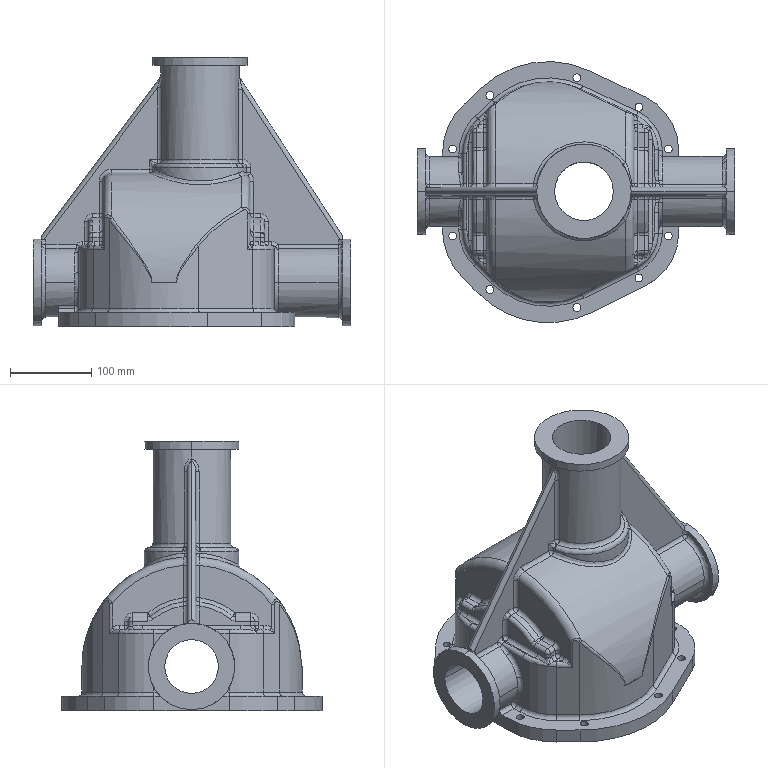Part | NX | features BREP 1 | 1 solid | 435 faces | box 389.177 x 320.4 x 330.766 mm | volume 3038683 mm3 | cylinder 193 | plane 87 | spline 73 | torus 44 | sphere 38 | commonest cylinder face diameters 10 x101 9.6 x20 29.6 x16 86 x6 66 x4 106 x4